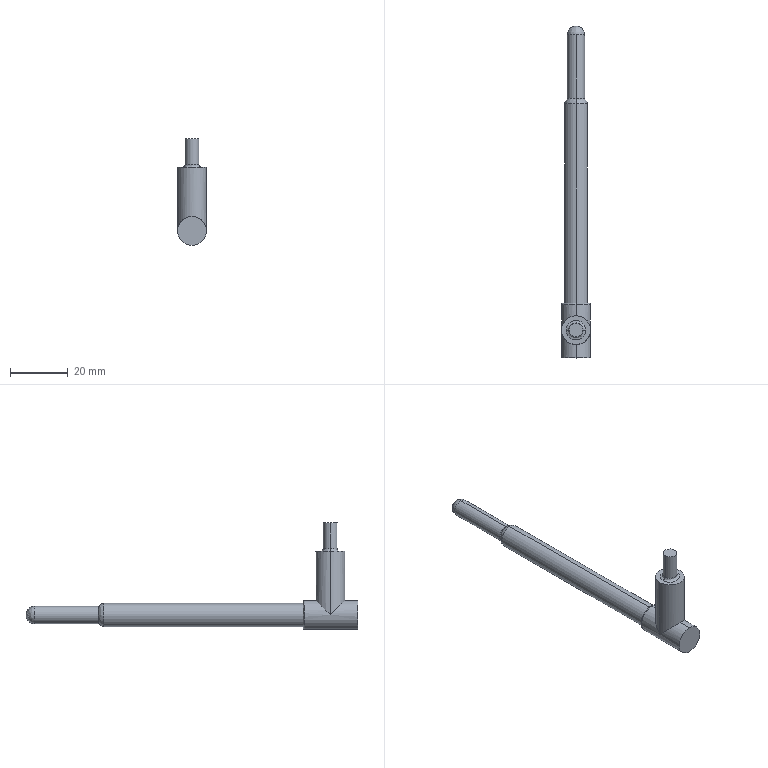Part | STEP file | 08 displacement_default | 1 solid | 22 faces | box 10 x 114.88 x 37 mm | volume 7298 mm3 | cylinder 10 | spline 7 | plane 5 | commonest cylinder face diameters 10 x4 4.8 x2 6 x2 8 x2